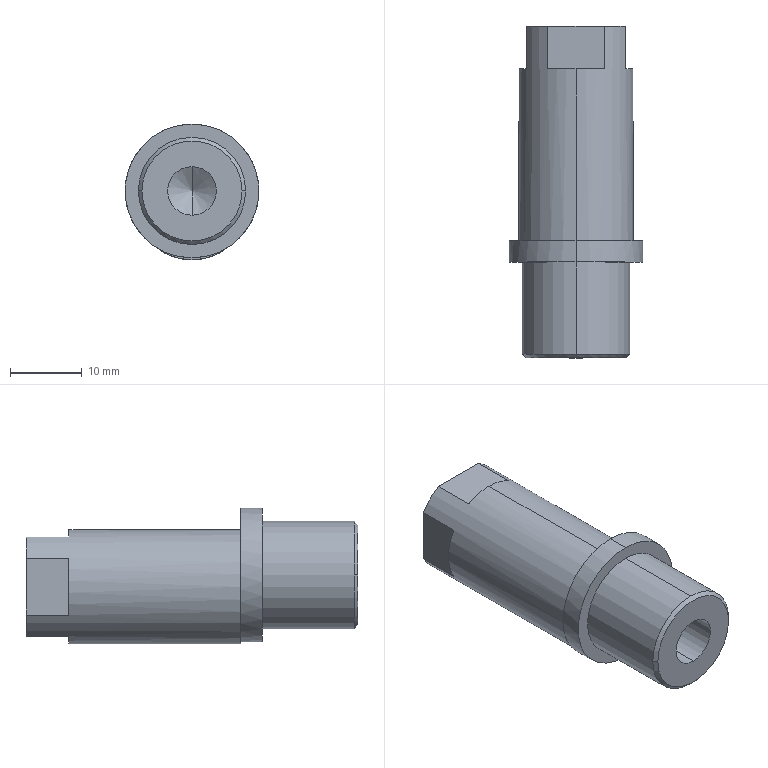Part | SolidWorks | features BaseBody 1 | 1 solid | 25 faces | box 18.7 x 46.4 x 19 mm | volume 8586 mm3 | plane 13 | cylinder 8 | cone 4 | commonest cylinder face diameters 6.8 x2 15 x2 16 x2 18.7 x2
STEP:
#1=CARTESIAN_POINT('',(3.962,27.,5.3));
#2=VERTEX_POINT('',#1);
#3=CARTESIAN_POINT('',(0.,27.,6.35));
#4=VERTEX_POINT('',#3);
#5=CARTESIAN_POINT('',(0.,27.,-1.65));
#6=DIRECTION('',(0.,-1.,0.));
#7=DIRECTION('',(0.,0.,-1.));
#8=AXIS2_PLACEMENT_3D('',#5,#6,#7);
#9=CIRCLE('',#8,8.);
#10=EDGE_CURVE('',#2,#4,#9,.T.);
#11=ORIENTED_EDGE('',*,*,#10,.T.);
#12=CARTESIAN_POINT('',(0.,3.,6.35));
#13=VERTEX_POINT('',#12);
#14=CARTESIAN_POINT('',(0.,33.,6.35));
#15=DIRECTION('',(0.,-1.,0.));
#16=VECTOR('',#15,1000.);
#17=LINE('',#14,#16);
#18=EDGE_CURVE('',#4,#13,#17,.T.);
#19=ORIENTED_EDGE('',*,*,#18,.T.);
#20=CARTESIAN_POINT('',(4.965,3.,-7.923));
#21=VERTEX_POINT('',#20);
#22=CARTESIAN_POINT('',(0.,3.,-1.65));
#23=DIRECTION('',(0.,1.,0.));
#24=DIRECTION('',(0.,0.,-1.));
#25=AXIS2_PLACEMENT_3D('',#22,#23,#24);
#26=CIRCLE('',#25,8.);
#27=EDGE_CURVE('',#13,#21,#26,.T.);
#28=ORIENTED_EDGE('',*,*,#27,.T.);
#29=CARTESIAN_POINT('',(0.,3.,-9.65));
#30=VERTEX_POINT('',#29);
#31=CARTESIAN_POINT('',(0.,3.,-1.65));
#32=DIRECTION('',(0.,1.,0.));
#33=DIRECTION('',(0.,0.,-1.));
#34=AXIS2_PLACEMENT_3D('',#31,#32,#33);
#35=CIRCLE('',#34,8.);
#36=EDGE_CURVE('',#21,#30,#35,.T.);
#37=ORIENTED_EDGE('',*,*,#36,.T.);
#38=CARTESIAN_POINT('',(0.,27.,-9.65));
#39=VERTEX_POINT('',#38);
#40=CARTESIAN_POINT('',(0.,33.,-9.65));
#41=DIRECTION('',(0.,-1.,0.));
#42=VECTOR('',#41,1000.);
#43=LINE('',#40,#42);
#44=EDGE_CURVE('',#39,#30,#43,.T.);
#45=ORIENTED_EDGE('',*,*,#44,.F.);
#46=CARTESIAN_POINT('',(3.962,27.,-8.6));
#47=VERTEX_POINT('',#46);
#48=CARTESIAN_POINT('',(0.,27.,-1.65));
#49=DIRECTION('',(0.,-1.,0.));
#50=DIRECTION('',(0.,0.,-1.));
#51=AXIS2_PLACEMENT_3D('',#48,#49,#50);
#52=CIRCLE('',#51,8.);
#53=EDGE_CURVE('',#39,#47,#52,.T.);
#54=ORIENTED_EDGE('',*,*,#53,.T.);
#55=CARTESIAN_POINT('',(3.962,33.,-8.6));
#56=VERTEX_POINT('',#55);
#57=CARTESIAN_POINT('',(3.962,33.,-8.6));
#58=DIRECTION('',(0.,1.,0.));
#59=VECTOR('',#58,1000.);
#60=LINE('',#57,#59);
#61=EDGE_CURVE('',#47,#56,#60,.T.);
#62=ORIENTED_EDGE('',*,*,#61,.T.);
#63=CARTESIAN_POINT('',(6.95,33.,-5.612));
#64=VERTEX_POINT('',#63);
#65=CARTESIAN_POINT('',(0.,33.,-1.65));
#66=DIRECTION('',(0.,-1.,0.));
#67=DIRECTION('',(0.,0.,-1.));
#68=AXIS2_PLACEMENT_3D('',#65,#66,#67);
#69=CIRCLE('',#68,8.);
#70=EDGE_CURVE('',#56,#64,#69,.T.);
#71=ORIENTED_EDGE('',*,*,#70,.T.);
#72=CARTESIAN_POINT('',(6.95,27.,-5.612));
#73=VERTEX_POINT('',#72);
#74=CARTESIAN_POINT('',(6.95,33.,-5.612));
#75=DIRECTION('',(0.,-1.,0.));
#76=VECTOR('',#75,1000.);
#77=LINE('',#74,#76);
#78=EDGE_CURVE('',#64,#73,#77,.T.);
#79=ORIENTED_EDGE('',*,*,#78,.T.);
#80=CARTESIAN_POINT('',(6.95,27.,2.312));
#81=VERTEX_POINT('',#80);
#82=CARTESIAN_POINT('',(0.,27.,-1.65));
#83=DIRECTION('',(0.,-1.,0.));
#84=DIRECTION('',(0.,0.,-1.));
#85=AXIS2_PLACEMENT_3D('',#82,#83,#84);
#86=CIRCLE('',#85,8.);
#87=EDGE_CURVE('',#73,#81,#86,.T.);
#88=ORIENTED_EDGE('',*,*,#87,.T.);
#89=CARTESIAN_POINT('',(6.95,33.,2.312));
#90=VERTEX_POINT('',#89);
#91=CARTESIAN_POINT('',(6.95,33.,2.312));
#92=DIRECTION('',(0.,1.,0.));
#93=VECTOR('',#92,1000.);
#94=LINE('',#91,#93);
#95=EDGE_CURVE('',#81,#90,#94,.T.);
#96=ORIENTED_EDGE('',*,*,#95,.T.);
#97=CARTESIAN_POINT('',(3.962,33.,5.3));
#98=VERTEX_POINT('',#97);
#99=CARTESIAN_POINT('',(0.,33.,-1.65));
#100=DIRECTION('',(0.,-1.,0.));
#101=DIRECTION('',(0.,0.,-1.));
#102=AXIS2_PLACEMENT_3D('',#99,#100,#101);
#103=CIRCLE('',#102,8.);
#104=EDGE_CURVE('',#90,#98,#103,.T.);
#105=ORIENTED_EDGE('',*,*,#104,.T.);
#106=CARTESIAN_POINT('',(3.962,33.,5.3));
#107=DIRECTION('',(0.,-1.,0.));
#108=VECTOR('',#107,1000.);
#109=LINE('',#106,#108);
#110=EDGE_CURVE('',#98,#2,#109,.T.);
#111=ORIENTED_EDGE('',*,*,#110,.T.);
#112=EDGE_LOOP('',(#11,#19,#28,#37,#45,#54,#62,#71,#79,#88,#96,#105,#111));
#113=FACE_OUTER_BOUND('',#112,.T.);
#114=CARTESIAN_POINT('',(0.,33.,-1.65));
#115=DIRECTION('',(0.,-1.,0.));
#116=DIRECTION('',(0.,0.,-1.));
#117=AXIS2_PLACEMENT_3D('',#114,#115,#116);
#118=CYLINDRICAL_SURFACE('',#117,8.);
#119=ADVANCED_FACE('',(#113),#118,.T.);
#120=CARTESIAN_POINT('',(0.,3.,9.35));
#121=VERTEX_POINT('',#120);
#122=CARTESIAN_POINT('',(0.,3.,0.));
#123=DIRECTION('',(0.,1.,0.));
#124=DIRECTION('',(0.,0.,-1.));
#125=AXIS2_PLACEMENT_3D('',#122,#123,#124);
#126=CIRCLE('',#125,9.35);
#127=EDGE_CURVE('',#121,#21,#126,.T.);
#128=ORIENTED_EDGE('',*,*,#127,.F.);
#129=CARTESIAN_POINT('',(0.,0.,9.35));
#130=VERTEX_POINT('',#129);
#131=CARTESIAN_POINT('',(0.,3.,9.35));
#132=DIRECTION('',(0.,-1.,0.));
#133=VECTOR('',#132,1000.);
#134=LINE('',#131,#133);
#135=EDGE_CURVE('',#121,#130,#134,.T.);
#136=ORIENTED_EDGE('',*,*,#135,.T.);
#137=CARTESIAN_POINT('',(0.,0.,-9.35));
#138=VERTEX_POINT('',#137);
#139=CARTESIAN_POINT('',(0.,0.,0.));
#140=DIRECTION('',(0.,1.,0.));
#141=DIRECTION('',(0.,0.,-1.));
#142=AXIS2_PLACEMENT_3D('',#139,#140,#141);
#143=CIRCLE('',#142,9.35);
#144=EDGE_CURVE('',#130,#138,#143,.T.);
#145=ORIENTED_EDGE('',*,*,#144,.T.);
#146=CARTESIAN_POINT('',(0.,3.,-9.35));
#147=VERTEX_POINT('',#146);
#148=CARTESIAN_POINT('',(0.,3.,-9.35));
#149=DIRECTION('',(0.,-1.,0.));
#150=VECTOR('',#149,1000.);
#151=LINE('',#148,#150);
#152=EDGE_CURVE('',#147,#138,#151,.T.);
#153=ORIENTED_EDGE('',*,*,#152,.F.);
#154=CARTESIAN_POINT('',(0.,3.,0.));
#155=DIRECTION('',(0.,-1.,0.));
#156=DIRECTION('',(0.,0.,-1.));
#157=AXIS2_PLACEMENT_3D('',#154,#155,#156);
#158=CIRCLE('',#157,9.35);
#159=EDGE_CURVE('',#147,#21,#158,.T.);
#160=ORIENTED_EDGE('',*,*,#159,.T.);
#161=EDGE_LOOP('',(#128,#136,#145,#153,#160));
#162=FACE_OUTER_BOUND('',#161,.T.);
#163=CARTESIAN_POINT('',(0.,3.,0.));
#164=DIRECTION('',(0.,-1.,0.));
#165=DIRECTION('',(0.,0.,-1.));
#166=AXIS2_PLACEMENT_3D('',#163,#164,#165);
#167=CYLINDRICAL_SURFACE('',#166,9.35);
#168=ADVANCED_FACE('',(#162),#167,.T.);
#169=CARTESIAN_POINT('',(7.5,-12.9,0.));
#170=VERTEX_POINT('',#169);
#171=CARTESIAN_POINT('',(0.,-12.9,-7.5));
#172=VERTEX_POINT('',#171);
#173=CARTESIAN_POINT('',(0.,-12.9,0.));
#174=DIRECTION('',(0.,1.,0.));
#175=DIRECTION('',(0.,0.,1.));
#176=AXIS2_PLACEMENT_3D('',#173,#174,#175);
#177=CIRCLE('',#176,7.5);
#178=EDGE_CURVE('',#170,#172,#177,.T.);
#179=ORIENTED_EDGE('',*,*,#178,.T.);
#180=CARTESIAN_POINT('',(0.,0.,-7.5));
#181=VERTEX_POINT('',#180);
#182=CARTESIAN_POINT('',(0.,-13.4,-7.5));
#183=DIRECTION('',(0.,1.,0.));
#184=VECTOR('',#183,1000.);
#185=LINE('',#182,#184);
#186=EDGE_CURVE('',#172,#181,#185,.T.);
#187=ORIENTED_EDGE('',*,*,#186,.T.);
#188=CARTESIAN_POINT('',(0.,0.,7.5));
#189=VERTEX_POINT('',#188);
#190=CARTESIAN_POINT('',(0.,0.,0.));
#191=DIRECTION('',(0.,-1.,0.));
#192=DIRECTION('',(0.,0.,1.));
#193=AXIS2_PLACEMENT_3D('',#190,#191,#192);
#194=CIRCLE('',#193,7.5);
#195=EDGE_CURVE('',#181,#189,#194,.T.);
#196=ORIENTED_EDGE('',*,*,#195,.T.);
#197=CARTESIAN_POINT('',(0.,-12.9,7.5));
#198=VERTEX_POINT('',#197);
#199=CARTESIAN_POINT('',(0.,-13.4,7.5));
#200=DIRECTION('',(0.,1.,0.));
#201=VECTOR('',#200,1000.);
#202=LINE('',#199,#201);
#203=EDGE_CURVE('',#198,#189,#202,.T.);
#204=ORIENTED_EDGE('',*,*,#203,.F.);
#205=CARTESIAN_POINT('',(0.,-12.9,0.));
#206=DIRECTION('',(0.,1.,0.));
#207=DIRECTION('',(0.,0.,1.));
#208=AXIS2_PLACEMENT_3D('',#205,#206,#207);
#209=CIRCLE('',#208,7.5);
#210=EDGE_CURVE('',#198,#170,#209,.T.);
#211=ORIENTED_EDGE('',*,*,#210,.T.);
#212=EDGE_LOOP('',(#179,#187,#196,#204,#211));
#213=FACE_OUTER_BOUND('',#212,.T.);
#214=CARTESIAN_POINT('',(0.,-13.4,0.));
#215=DIRECTION('',(0.,1.,0.));
#216=DIRECTION('',(0.,0.,1.));
#217=AXIS2_PLACEMENT_3D('',#214,#215,#216);
#218=CYLINDRICAL_SURFACE('',#217,7.5);
#219=ADVANCED_FACE('',(#213),#218,.T.);
#220=CARTESIAN_POINT('',(-7.,-13.4,0.));
#221=VERTEX_POINT('',#220);
#222=CARTESIAN_POINT('',(7.,-13.4,0.));
#223=VERTEX_POINT('',#222);
#224=CARTESIAN_POINT('',(0.,-13.4,0.));
#225=DIRECTION('',(0.,1.,0.));
#226=DIRECTION('',(-1.,0.,0.));
#227=AXIS2_PLACEMENT_3D('',#224,#225,#226);
#228=CIRCLE('',#227,7.);
#229=EDGE_CURVE('',#221,#223,#228,.T.);
#230=ORIENTED_EDGE('',*,*,#229,.T.);
#231=CARTESIAN_POINT('',(7.5,-12.9,0.));
#232=DIRECTION('',(0.7071,0.7071,0.));
#233=VECTOR('',#232,1000.);
#234=LINE('',#231,#233);
#235=EDGE_CURVE('',#223,#170,#234,.T.);
#236=ORIENTED_EDGE('',*,*,#235,.T.);
#237=ORIENTED_EDGE('',*,*,#210,.F.);
#238=CARTESIAN_POINT('',(-7.5,-12.9,0.));
#239=VERTEX_POINT('',#238);
#240=CARTESIAN_POINT('',(0.,-12.9,0.));
#241=DIRECTION('',(0.,1.,0.));
#242=DIRECTION('',(0.,0.,1.));
#243=AXIS2_PLACEMENT_3D('',#240,#241,#242);
#244=CIRCLE('',#243,7.5);
#245=EDGE_CURVE('',#239,#198,#244,.T.);
#246=ORIENTED_EDGE('',*,*,#245,.F.);
#247=CARTESIAN_POINT('',(-7.5,-12.9,0.));
#248=DIRECTION('',(-0.7071,0.7071,0.));
#249=VECTOR('',#248,1000.);
#250=LINE('',#247,#249);
#251=EDGE_CURVE('',#221,#239,#250,.T.);
#252=ORIENTED_EDGE('',*,*,#251,.F.);
#253=EDGE_LOOP('',(#230,#236,#237,#246,#252));
#254=FACE_OUTER_BOUND('',#253,.T.);
#255=CARTESIAN_POINT('',(0.,-12.9,0.));
#256=DIRECTION('',(0.,1.,0.));
#257=DIRECTION('',(-1.,0.,0.));
#258=AXIS2_PLACEMENT_3D('',#255,#256,#257);
#259=CONICAL_SURFACE('',#258,7.5,0.7854);
#260=ADVANCED_FACE('',(#254),#259,.T.);
#261=CARTESIAN_POINT('',(0.,-0.4,3.4));
#262=VERTEX_POINT('',#261);
#263=CARTESIAN_POINT('',(0.,-0.4,-3.4));
#264=VERTEX_POINT('',#263);
#265=CARTESIAN_POINT('',(0.,-0.4,0.));
#266=DIRECTION('',(0.,-1.,0.));
#267=DIRECTION('',(0.,0.,-1.));
#268=AXIS2_PLACEMENT_3D('',#265,#266,#267);
#269=CIRCLE('',#268,3.4);
#270=EDGE_CURVE('',#262,#264,#269,.T.);
#271=ORIENTED_EDGE('',*,*,#270,.F.);
#272=CARTESIAN_POINT('',(0.,-13.4,3.4));
#273=VERTEX_POINT('',#272);
#274=CARTESIAN_POINT('',(0.,-13.4,3.4));
#275=DIRECTION('',(0.,-1.,0.));
#276=VECTOR('',#275,1000.);
#277=LINE('',#274,#276);
#278=EDGE_CURVE('',#262,#273,#277,.T.);
#279=ORIENTED_EDGE('',*,*,#278,.T.);
#280=CARTESIAN_POINT('',(0.,-13.4,-3.4));
#281=VERTEX_POINT('',#280);
#282=CARTESIAN_POINT('',(0.,-13.4,0.));
#283=DIRECTION('',(0.,1.,0.));
#284=DIRECTION('',(0.,0.,-1.));
#285=AXIS2_PLACEMENT_3D('',#282,#283,#284);
#286=CIRCLE('',#285,3.4);
#287=EDGE_CURVE('',#281,#273,#286,.T.);
#288=ORIENTED_EDGE('',*,*,#287,.F.);
#289=CARTESIAN_POINT('',(0.,-13.4,-3.4));
#290=DIRECTION('',(0.,-1.,0.));
#291=VECTOR('',#290,1000.);
#292=LINE('',#289,#291);
#293=EDGE_CURVE('',#264,#281,#292,.T.);
#294=ORIENTED_EDGE('',*,*,#293,.F.);
#295=EDGE_LOOP('',(#271,#279,#288,#294));
#296=FACE_OUTER_BOUND('',#295,.T.);
#297=CARTESIAN_POINT('',(0.,-13.4,0.));
#298=DIRECTION('',(0.,-1.,0.));
#299=DIRECTION('',(0.,0.,-1.));
#300=AXIS2_PLACEMENT_3D('',#297,#298,#299);
#301=CYLINDRICAL_SURFACE('',#300,3.4);
#302=ADVANCED_FACE('',(#296),#301,.F.);
#303=CARTESIAN_POINT('',(0.,1.643,0.));
#304=VERTEX_POINT('',#303);
#305=CARTESIAN_POINT('',(0.,-0.4,-3.4));
#306=DIRECTION('',(0.,-0.515,-0.8572));
#307=VECTOR('',#306,1000.);
#308=LINE('',#305,#307);
#309=EDGE_CURVE('',#304,#264,#308,.T.);
#310=ORIENTED_EDGE('',*,*,#309,.F.);
#311=CARTESIAN_POINT('',(0.,-0.4,3.4));
#312=DIRECTION('',(0.,-0.515,0.8572));
#313=VECTOR('',#312,1000.);
#314=LINE('',#311,#313);
#315=EDGE_CURVE('',#304,#262,#314,.T.);
#316=ORIENTED_EDGE('',*,*,#315,.T.);
#317=ORIENTED_EDGE('',*,*,#270,.T.);
#318=EDGE_LOOP('',(#310,#316,#317));
#319=FACE_OUTER_BOUND('',#318,.T.);
#320=CARTESIAN_POINT('',(0.,-0.4,0.));
#321=DIRECTION('',(0.,-1.,0.));
#322=DIRECTION('',(0.,0.,-1.));
#323=AXIS2_PLACEMENT_3D('',#320,#321,#322);
#324=CONICAL_SURFACE('',#323,3.4,1.03);
#325=ADVANCED_FACE('',(#319),#324,.F.);
#326=ORIENTED_EDGE('',*,*,#18,.F.);
#327=CARTESIAN_POINT('',(-3.962,27.,5.3));
#328=VERTEX_POINT('',#327);
#329=CARTESIAN_POINT('',(0.,27.,-1.65));
#330=DIRECTION('',(0.,-1.,0.));
#331=DIRECTION('',(0.,0.,-1.));
#332=AXIS2_PLACEMENT_3D('',#329,#330,#331);
#333=CIRCLE('',#332,8.);
#334=EDGE_CURVE('',#4,#328,#333,.T.);
#335=ORIENTED_EDGE('',*,*,#334,.T.);
#336=CARTESIAN_POINT('',(-3.962,33.,5.3));
#337=VERTEX_POINT('',#336);
#338=CARTESIAN_POINT('',(-3.962,27.,5.3));
#339=DIRECTION('',(0.,-1.,0.));
#340=VECTOR('',#339,1000.);
#341=LINE('',#338,#340);
#342=EDGE_CURVE('',#337,#328,#341,.T.);
#343=ORIENTED_EDGE('',*,*,#342,.F.);
#344=CARTESIAN_POINT('',(-6.95,33.,2.312));
#345=VERTEX_POINT('',#344);
#346=CARTESIAN_POINT('',(0.,33.,-1.65));
#347=DIRECTION('',(0.,1.,0.));
#348=DIRECTION('',(0.,0.,-1.));
#349=AXIS2_PLACEMENT_3D('',#346,#347,#348);
#350=CIRCLE('',#349,8.);
#351=EDGE_CURVE('',#345,#337,#350,.T.);
#352=ORIENTED_EDGE('',*,*,#351,.F.);
#353=CARTESIAN_POINT('',(-6.95,27.,2.312));
#354=VERTEX_POINT('',#353);
#355=CARTESIAN_POINT('',(-6.95,33.,2.312));
#356=DIRECTION('',(0.,-1.,0.));
#357=VECTOR('',#356,1000.);
#358=LINE('',#355,#357);
#359=EDGE_CURVE('',#345,#354,#358,.T.);
#360=ORIENTED_EDGE('',*,*,#359,.T.);
#361=CARTESIAN_POINT('',(-6.95,27.,-5.612));
#362=VERTEX_POINT('',#361);
#363=CARTESIAN_POINT('',(0.,27.,-1.65));
#364=DIRECTION('',(0.,-1.,0.));
#365=DIRECTION('',(0.,0.,-1.));
#366=AXIS2_PLACEMENT_3D('',#363,#364,#365);
#367=CIRCLE('',#366,8.);
#368=EDGE_CURVE('',#354,#362,#367,.T.);
#369=ORIENTED_EDGE('',*,*,#368,.T.);
#370=CARTESIAN_POINT('',(-6.95,33.,-5.612));
#371=VERTEX_POINT('',#370);
#372=CARTESIAN_POINT('',(-6.95,33.,-5.612));
#373=DIRECTION('',(0.,1.,0.));
#374=VECTOR('',#373,1000.);
#375=LINE('',#372,#374);
#376=EDGE_CURVE('',#362,#371,#375,.T.);
#377=ORIENTED_EDGE('',*,*,#376,.T.);
#378=CARTESIAN_POINT('',(-3.962,33.,-8.6));
#379=VERTEX_POINT('',#378);
#380=CARTESIAN_POINT('',(0.,33.,-1.65));
#381=DIRECTION('',(0.,1.,0.));
#382=DIRECTION('',(0.,0.,-1.));
#383=AXIS2_PLACEMENT_3D('',#380,#381,#382);
#384=CIRCLE('',#383,8.);
#385=EDGE_CURVE('',#379,#371,#384,.T.);
#386=ORIENTED_EDGE('',*,*,#385,.F.);
#387=CARTESIAN_POINT('',(-3.962,27.,-8.6));
#388=VERTEX_POINT('',#387);
#389=CARTESIAN_POINT('',(-3.962,27.,-8.6));
#390=DIRECTION('',(0.,-1.,0.));
#391=VECTOR('',#390,1000.);
#392=LINE('',#389,#391);
#393=EDGE_CURVE('',#379,#388,#392,.T.);
#394=ORIENTED_EDGE('',*,*,#393,.T.);
#395=CARTESIAN_POINT('',(0.,27.,-1.65));
#396=DIRECTION('',(0.,-1.,0.));
#397=DIRECTION('',(0.,0.,-1.));
#398=AXIS2_PLACEMENT_3D('',#395,#396,#397);
#399=CIRCLE('',#398,8.);
#400=EDGE_CURVE('',#388,#39,#399,.T.);
#401=ORIENTED_EDGE('',*,*,#400,.T.);
#402=ORIENTED_EDGE('',*,*,#44,.T.);
#403=CARTESIAN_POINT('',(-4.965,3.,-7.923));
#404=VERTEX_POINT('',#403);
#405=CARTESIAN_POINT('',(0.,3.,-1.65));
#406=DIRECTION('',(0.,1.,0.));
#407=DIRECTION('',(0.,0.,-1.));
#408=AXIS2_PLACEMENT_3D('',#405,#406,#407);
#409=CIRCLE('',#408,8.);
#410=EDGE_CURVE('',#30,#404,#409,.T.);
#411=ORIENTED_EDGE('',*,*,#410,.T.);
#412=CARTESIAN_POINT('',(0.,3.,-1.65));
#413=DIRECTION('',(0.,1.,0.));
#414=DIRECTION('',(0.,0.,-1.));
#415=AXIS2_PLACEMENT_3D('',#412,#413,#414);
#416=CIRCLE('',#415,8.);
#417=EDGE_CURVE('',#404,#13,#416,.T.);
#418=ORIENTED_EDGE('',*,*,#417,.T.);
#419=EDGE_LOOP('',(#326,#335,#343,#352,#360,#369,#377,#386,#394,#401,#402,#411,#418));
#420=FACE_OUTER_BOUND('',#419,.T.);
#421=CARTESIAN_POINT('',(0.,33.,-1.65));
#422=DIRECTION('',(0.,-1.,0.));
#423=DIRECTION('',(0.,0.,-1.));
#424=AXIS2_PLACEMENT_3D('',#421,#422,#423);
#425=CYLINDRICAL_SURFACE('',#424,8.);
#426=ADVANCED_FACE('',(#420),#425,.T.);
#427=ORIENTED_EDGE('',*,*,#110,.F.);
#428=CARTESIAN_POINT('',(-6.95,33.,5.3));
#429=DIRECTION('',(-1.,0.,0.));
#430=VECTOR('',#429,1000.);
#431=LINE('',#428,#430);
#432=EDGE_CURVE('',#98,#337,#431,.T.);
#433=ORIENTED_EDGE('',*,*,#432,.T.);
#434=ORIENTED_EDGE('',*,*,#342,.T.);
#435=CARTESIAN_POINT('',(-6.95,27.,5.3));
#436=DIRECTION('',(1.,0.,0.));
#437=VECTOR('',#436,1000.);
#438=LINE('',#435,#437);
#439=EDGE_CURVE('',#328,#2,#438,.T.);
#440=ORIENTED_EDGE('',*,*,#439,.T.);
#441=EDGE_LOOP('',(#427,#433,#434,#440));
#442=FACE_OUTER_BOUND('',#441,.T.);
#443=CARTESIAN_POINT('',(-6.95,27.,5.3));
#444=DIRECTION('',(0.,0.,1.));
#445=DIRECTION('',(1.,0.,0.));
#446=AXIS2_PLACEMENT_3D('',#443,#444,#445);
#447=PLANE('',#446);
#448=ADVANCED_FACE('',(#442),#447,.T.);
#449=CARTESIAN_POINT('',(6.95,33.,-1.65));
#450=DIRECTION('',(0.,0.,-1.));
#451=VECTOR('',#450,1000.);
#452=LINE('',#449,#451);
#453=EDGE_CURVE('',#90,#64,#452,.T.);
#454=ORIENTED_EDGE('',*,*,#453,.T.);
#455=ORIENTED_EDGE('',*,*,#70,.F.);
#456=CARTESIAN_POINT('',(0.,33.,-8.6));
#457=DIRECTION('',(-1.,0.,0.));
#458=VECTOR('',#457,1000.);
#459=LINE('',#456,#458);
#460=EDGE_CURVE('',#56,#379,#459,.T.);
#461=ORIENTED_EDGE('',*,*,#460,.T.);
#462=ORIENTED_EDGE('',*,*,#385,.T.);
#463=CARTESIAN_POINT('',(-6.95,33.,-1.65));
#464=DIRECTION('',(0.,0.,1.));
#465=VECTOR('',#464,1000.);
#466=LINE('',#463,#465);
#467=EDGE_CURVE('',#371,#345,#466,.T.);
#468=ORIENTED_EDGE('',*,*,#467,.T.);
#469=ORIENTED_EDGE('',*,*,#351,.T.);
#470=ORIENTED_EDGE('',*,*,#432,.F.);
#471=ORIENTED_EDGE('',*,*,#104,.F.);
#472=EDGE_LOOP('',(#454,#455,#461,#462,#468,#469,#470,#471));
#473=FACE_OUTER_BOUND('',#472,.T.);
#474=CARTESIAN_POINT('',(0.,33.,-1.65));
#475=DIRECTION('',(0.,1.,0.));
#476=DIRECTION('',(0.,0.,1.));
#477=AXIS2_PLACEMENT_3D('',#474,#475,#476);
#478=PLANE('',#477);
#479=ADVANCED_FACE('',(#473),#478,.T.);
#480=ORIENTED_EDGE('',*,*,#95,.F.);
#481=CARTESIAN_POINT('',(6.95,27.,-8.6));
#482=DIRECTION('',(0.,0.,1.));
#483=VECTOR('',#482,1000.);
#484=LINE('',#481,#483);
#485=EDGE_CURVE('',#73,#81,#484,.T.);
#486=ORIENTED_EDGE('',*,*,#485,.F.);
#487=ORIENTED_EDGE('',*,*,#78,.F.);
#488=ORIENTED_EDGE('',*,*,#453,.F.);
#489=EDGE_LOOP('',(#480,#486,#487,#488));
#490=FACE_OUTER_BOUND('',#489,.T.);
#491=CARTESIAN_POINT('',(6.95,27.,-8.6));
#492=DIRECTION('',(-1.,0.,0.));
#493=DIRECTION('',(0.,0.,1.));
#494=AXIS2_PLACEMENT_3D('',#491,#492,#493);
#495=PLANE('',#494);
#496=ADVANCED_FACE('',(#490),#495,.F.);
#497=ORIENTED_EDGE('',*,*,#87,.F.);
#498=ORIENTED_EDGE('',*,*,#485,.T.);
#499=EDGE_LOOP('',(#497,#498));
#500=FACE_OUTER_BOUND('',#499,.T.);
#501=CARTESIAN_POINT('',(0.,27.,-0.15));
#502=DIRECTION('',(0.,1.,0.));
#503=DIRECTION('',(0.,0.,1.));
#504=AXIS2_PLACEMENT_3D('',#501,#502,#503);
#505=PLANE('',#504);
#506=ADVANCED_FACE('',(#500),#505,.T.);
#507=ORIENTED_EDGE('',*,*,#61,.F.);
#508=CARTESIAN_POINT('',(-6.95,27.,-8.6));
#509=DIRECTION('',(1.,0.,0.));
#510=VECTOR('',#509,1000.);
#511=LINE('',#508,#510);
#512=EDGE_CURVE('',#388,#47,#511,.T.);
#513=ORIENTED_EDGE('',*,*,#512,.F.);
#514=ORIENTED_EDGE('',*,*,#393,.F.);
#515=ORIENTED_EDGE('',*,*,#460,.F.);
#516=EDGE_LOOP('',(#507,#513,#514,#515));
#517=FACE_OUTER_BOUND('',#516,.T.);
#518=CARTESIAN_POINT('',(-6.95,27.,-8.6));
#519=DIRECTION('',(0.,0.,1.));
#520=DIRECTION('',(1.,0.,0.));
#521=AXIS2_PLACEMENT_3D('',#518,#519,#520);
#522=PLANE('',#521);
#523=ADVANCED_FACE('',(#517),#522,.F.);
#524=ORIENTED_EDGE('',*,*,#400,.F.);
#525=ORIENTED_EDGE('',*,*,#512,.T.);
#526=ORIENTED_EDGE('',*,*,#53,.F.);
#527=EDGE_LOOP('',(#524,#525,#526));
#528=FACE_OUTER_BOUND('',#527,.T.);
#529=CARTESIAN_POINT('',(0.,27.,-0.15));
#530=DIRECTION('',(0.,1.,0.));
#531=DIRECTION('',(0.,0.,1.));
#532=AXIS2_PLACEMENT_3D('',#529,#530,#531);
#533=PLANE('',#532);
#534=ADVANCED_FACE('',(#528),#533,.T.);
#535=CARTESIAN_POINT('',(0.,3.,0.));
#536=DIRECTION('',(0.,-1.,0.));
#537=DIRECTION('',(0.,0.,-1.));
#538=AXIS2_PLACEMENT_3D('',#535,#536,#537);
#539=CIRCLE('',#538,9.35);
#540=EDGE_CURVE('',#404,#147,#539,.T.);
#541=ORIENTED_EDGE('',*,*,#540,.F.);
#542=ORIENTED_EDGE('',*,*,#410,.F.);
#543=ORIENTED_EDGE('',*,*,#36,.F.);
#544=ORIENTED_EDGE('',*,*,#159,.F.);
#545=EDGE_LOOP('',(#541,#542,#543,#544));
#546=FACE_OUTER_BOUND('',#545,.T.);
#547=CARTESIAN_POINT('',(0.,3.,-1.65));
#548=DIRECTION('',(0.,1.,0.));
#549=DIRECTION('',(0.,0.,1.));
#550=AXIS2_PLACEMENT_3D('',#547,#548,#549);
#551=PLANE('',#550);
#552=ADVANCED_FACE('',(#546),#551,.F.);
#553=CARTESIAN_POINT('',(0.,3.,0.));
#554=DIRECTION('',(0.,1.,0.));
#555=DIRECTION('',(0.,0.,-1.));
#556=AXIS2_PLACEMENT_3D('',#553,#554,#555);
#557=CIRCLE('',#556,9.35);
#558=EDGE_CURVE('',#404,#121,#557,.T.);
#559=ORIENTED_EDGE('',*,*,#558,.T.);
#560=ORIENTED_EDGE('',*,*,#127,.T.);
#561=ORIENTED_EDGE('',*,*,#27,.F.);
#562=ORIENTED_EDGE('',*,*,#417,.F.);
#563=EDGE_LOOP('',(#559,#560,#561,#562));
#564=FACE_OUTER_BOUND('',#563,.T.);
#565=CARTESIAN_POINT('',(0.,3.,0.));
#566=DIRECTION('',(0.,1.,0.));
#567=DIRECTION('',(0.,0.,1.));
#568=AXIS2_PLACEMENT_3D('',#565,#566,#567);
#569=PLANE('',#568);
#570=ADVANCED_FACE('',(#564),#569,.T.);
#571=ORIENTED_EDGE('',*,*,#10,.F.);
#572=ORIENTED_EDGE('',*,*,#439,.F.);
#573=ORIENTED_EDGE('',*,*,#334,.F.);
#574=EDGE_LOOP('',(#571,#572,#573));
#575=FACE_OUTER_BOUND('',#574,.T.);
#576=CARTESIAN_POINT('',(0.,27.,-0.15));
#577=DIRECTION('',(0.,1.,0.));
#578=DIRECTION('',(0.,0.,1.));
#579=AXIS2_PLACEMENT_3D('',#576,#577,#578);
#580=PLANE('',#579);
#581=ADVANCED_FACE('',(#575),#580,.T.);
#582=ORIENTED_EDGE('',*,*,#359,.F.);
#583=ORIENTED_EDGE('',*,*,#467,.F.);
#584=ORIENTED_EDGE('',*,*,#376,.F.);
#585=CARTESIAN_POINT('',(-6.95,27.,-8.6));
#586=DIRECTION('',(0.,0.,1.));
#587=VECTOR('',#586,1000.);
#588=LINE('',#585,#587);
#589=EDGE_CURVE('',#362,#354,#588,.T.);
#590=ORIENTED_EDGE('',*,*,#589,.T.);
#591=EDGE_LOOP('',(#582,#583,#584,#590));
#592=FACE_OUTER_BOUND('',#591,.T.);
#593=CARTESIAN_POINT('',(-6.95,27.,-8.6));
#594=DIRECTION('',(-1.,0.,0.));
#595=DIRECTION('',(0.,0.,1.));
#596=AXIS2_PLACEMENT_3D('',#593,#594,#595);
#597=PLANE('',#596);
#598=ADVANCED_FACE('',(#592),#597,.T.);
#599=ORIENTED_EDGE('',*,*,#368,.F.);
#600=ORIENTED_EDGE('',*,*,#589,.F.);
#601=EDGE_LOOP('',(#599,#600));
#602=FACE_OUTER_BOUND('',#601,.T.);
#603=CARTESIAN_POINT('',(0.,27.,-0.15));
#604=DIRECTION('',(0.,1.,0.));
#605=DIRECTION('',(0.,0.,1.));
#606=AXIS2_PLACEMENT_3D('',#603,#604,#605);
#607=PLANE('',#606);
#608=ADVANCED_FACE('',(#602),#607,.T.);
#609=ORIENTED_EDGE('',*,*,#135,.F.);
#610=ORIENTED_EDGE('',*,*,#558,.F.);
#611=ORIENTED_EDGE('',*,*,#540,.T.);
#612=ORIENTED_EDGE('',*,*,#152,.T.);
#613=CARTESIAN_POINT('',(0.,0.,0.));
#614=DIRECTION('',(0.,1.,0.));
#615=DIRECTION('',(0.,0.,-1.));
#616=AXIS2_PLACEMENT_3D('',#613,#614,#615);
#617=CIRCLE('',#616,9.35);
#618=EDGE_CURVE('',#138,#130,#617,.T.);
#619=ORIENTED_EDGE('',*,*,#618,.T.);
#620=EDGE_LOOP('',(#609,#610,#611,#612,#619));
#621=FACE_OUTER_BOUND('',#620,.T.);
#622=CARTESIAN_POINT('',(0.,3.,0.));
#623=DIRECTION('',(0.,-1.,0.));
#624=DIRECTION('',(0.,0.,-1.));
#625=AXIS2_PLACEMENT_3D('',#622,#623,#624);
#626=CYLINDRICAL_SURFACE('',#625,9.35);
#627=ADVANCED_FACE('',(#621),#626,.T.);
#628=ORIENTED_EDGE('',*,*,#618,.F.);
#629=ORIENTED_EDGE('',*,*,#144,.F.);
#630=EDGE_LOOP('',(#628,#629));
#631=FACE_OUTER_BOUND('',#630,.T.);
#632=CARTESIAN_POINT('',(0.,0.,0.));
#633=DIRECTION('',(0.,-1.,0.));
#634=DIRECTION('',(0.,0.,1.));
#635=AXIS2_PLACEMENT_3D('',#632,#633,#634);
#636=CIRCLE('',#635,7.5);
#637=EDGE_CURVE('',#189,#181,#636,.T.);
#638=ORIENTED_EDGE('',*,*,#637,.F.);
#639=ORIENTED_EDGE('',*,*,#195,.F.);
#640=EDGE_LOOP('',(#638,#639));
#641=FACE_BOUND('',#640,.T.);
#642=CARTESIAN_POINT('',(0.,0.,0.));
#643=DIRECTION('',(0.,1.,0.));
#644=DIRECTION('',(0.,0.,1.));
#645=AXIS2_PLACEMENT_3D('',#642,#643,#644);
#646=PLANE('',#645);
#647=ADVANCED_FACE('',(#631,#641),#646,.F.);
#648=ORIENTED_EDGE('',*,*,#186,.F.);
#649=CARTESIAN_POINT('',(0.,-12.9,0.));
#650=DIRECTION('',(0.,1.,0.));
#651=DIRECTION('',(0.,0.,1.));
#652=AXIS2_PLACEMENT_3D('',#649,#650,#651);
#653=CIRCLE('',#652,7.5);
#654=EDGE_CURVE('',#172,#239,#653,.T.);
#655=ORIENTED_EDGE('',*,*,#654,.T.);
#656=ORIENTED_EDGE('',*,*,#245,.T.);
#657=ORIENTED_EDGE('',*,*,#203,.T.);
#658=ORIENTED_EDGE('',*,*,#637,.T.);
#659=EDGE_LOOP('',(#648,#655,#656,#657,#658));
#660=FACE_OUTER_BOUND('',#659,.T.);
#661=CARTESIAN_POINT('',(0.,-13.4,0.));
#662=DIRECTION('',(0.,1.,0.));
#663=DIRECTION('',(0.,0.,1.));
#664=AXIS2_PLACEMENT_3D('',#661,#662,#663);
#665=CYLINDRICAL_SURFACE('',#664,7.5);
#666=ADVANCED_FACE('',(#660),#665,.T.);
#667=ORIENTED_EDGE('',*,*,#235,.F.);
#668=CARTESIAN_POINT('',(0.,-13.4,0.));
#669=DIRECTION('',(0.,1.,0.));
#670=DIRECTION('',(-1.,0.,0.));
#671=AXIS2_PLACEMENT_3D('',#668,#669,#670);
#672=CIRCLE('',#671,7.);
#673=EDGE_CURVE('',#223,#221,#672,.T.);
#674=ORIENTED_EDGE('',*,*,#673,.T.);
#675=ORIENTED_EDGE('',*,*,#251,.T.);
#676=ORIENTED_EDGE('',*,*,#654,.F.);
#677=ORIENTED_EDGE('',*,*,#178,.F.);
#678=EDGE_LOOP('',(#667,#674,#675,#676,#677));
#679=FACE_OUTER_BOUND('',#678,.T.);
#680=CARTESIAN_POINT('',(0.,-12.9,0.));
#681=DIRECTION('',(0.,1.,0.));
#682=DIRECTION('',(-1.,0.,0.));
#683=AXIS2_PLACEMENT_3D('',#680,#681,#682);
#684=CONICAL_SURFACE('',#683,7.5,0.7854);
#685=ADVANCED_FACE('',(#679),#684,.T.);
#686=ORIENTED_EDGE('',*,*,#287,.T.);
#687=CARTESIAN_POINT('',(0.,-13.4,0.));
#688=DIRECTION('',(0.,1.,0.));
#689=DIRECTION('',(0.,0.,-1.));
#690=AXIS2_PLACEMENT_3D('',#687,#688,#689);
#691=CIRCLE('',#690,3.4);
#692=EDGE_CURVE('',#273,#281,#691,.T.);
#693=ORIENTED_EDGE('',*,*,#692,.T.);
#694=EDGE_LOOP('',(#686,#693));
#695=FACE_BOUND('',#694,.T.);
#696=ORIENTED_EDGE('',*,*,#229,.F.);
#697=ORIENTED_EDGE('',*,*,#673,.F.);
#698=EDGE_LOOP('',(#696,#697));
#699=FACE_OUTER_BOUND('',#698,.T.);
#700=CARTESIAN_POINT('',(0.,-13.4,0.));
#701=DIRECTION('',(0.,-1.,0.));
#702=DIRECTION('',(0.,0.,-1.));
#703=AXIS2_PLACEMENT_3D('',#700,#701,#702);
#704=PLANE('',#703);
#705=ADVANCED_FACE('',(#695,#699),#704,.T.);
#706=ORIENTED_EDGE('',*,*,#278,.F.);
#707=CARTESIAN_POINT('',(0.,-0.4,0.));
#708=DIRECTION('',(0.,-1.,0.));
#709=DIRECTION('',(0.,0.,-1.));
#710=AXIS2_PLACEMENT_3D('',#707,#708,#709);
#711=CIRCLE('',#710,3.4);
#712=EDGE_CURVE('',#264,#262,#711,.T.);
#713=ORIENTED_EDGE('',*,*,#712,.F.);
#714=ORIENTED_EDGE('',*,*,#293,.T.);
#715=ORIENTED_EDGE('',*,*,#692,.F.);
#716=EDGE_LOOP('',(#706,#713,#714,#715));
#717=FACE_OUTER_BOUND('',#716,.T.);
#718=CARTESIAN_POINT('',(0.,-13.4,0.));
#719=DIRECTION('',(0.,-1.,0.));
#720=DIRECTION('',(0.,0.,-1.));
#721=AXIS2_PLACEMENT_3D('',#718,#719,#720);
#722=CYLINDRICAL_SURFACE('',#721,3.4);
#723=ADVANCED_FACE('',(#717),#722,.F.);
#724=ORIENTED_EDGE('',*,*,#315,.F.);
#725=ORIENTED_EDGE('',*,*,#309,.T.);
#726=ORIENTED_EDGE('',*,*,#712,.T.);
#727=EDGE_LOOP('',(#724,#725,#726));
#728=FACE_OUTER_BOUND('',#727,.T.);
#729=CARTESIAN_POINT('',(0.,-0.4,0.));
#730=DIRECTION('',(0.,-1.,0.));
#731=DIRECTION('',(0.,0.,-1.));
#732=AXIS2_PLACEMENT_3D('',#729,#730,#731);
#733=CONICAL_SURFACE('',#732,3.4,1.03);
#734=ADVANCED_FACE('',(#728),#733,.F.);
#735=CLOSED_SHELL('',(#119,#168,#219,#260,#302,#325,#426,#448,#479,#496,#506,#523,#534,#552,#570,#581,#598,#608,#627,#647,#666,#685,#705,#723,#734));
#736=MANIFOLD_SOLID_BREP('',#735);
#737=CARTESIAN_POINT('',(0.,0.,0.));
#738=DIRECTION('',(0.,0.,1.));
#739=DIRECTION('',(1.,0.,0.));
#740=AXIS2_PLACEMENT_3D('',#737,#738,#739);
#741=(LENGTH_UNIT()NAMED_UNIT(*)SI_UNIT(.MILLI.,.METRE.));
#742=UNCERTAINTY_MEASURE_WITH_UNIT(LENGTH_MEASURE(0.00001),#741,'','');
#743=(NAMED_UNIT(*)PLANE_ANGLE_UNIT()SI_UNIT($,.RADIAN.));
#744=(NAMED_UNIT(*)SI_UNIT($,.STERADIAN.)SOLID_ANGLE_UNIT());
#745=(GEOMETRIC_REPRESENTATION_CONTEXT(3)GLOBAL_UNCERTAINTY_ASSIGNED_CONTEXT((#742))GLOBAL_UNIT_ASSIGNED_CONTEXT((#741,#743,#744))REPRESENTATION_CONTEXT('',''));
#746=ADVANCED_BREP_SHAPE_REPRESENTATION('',(#736,#740),#745);